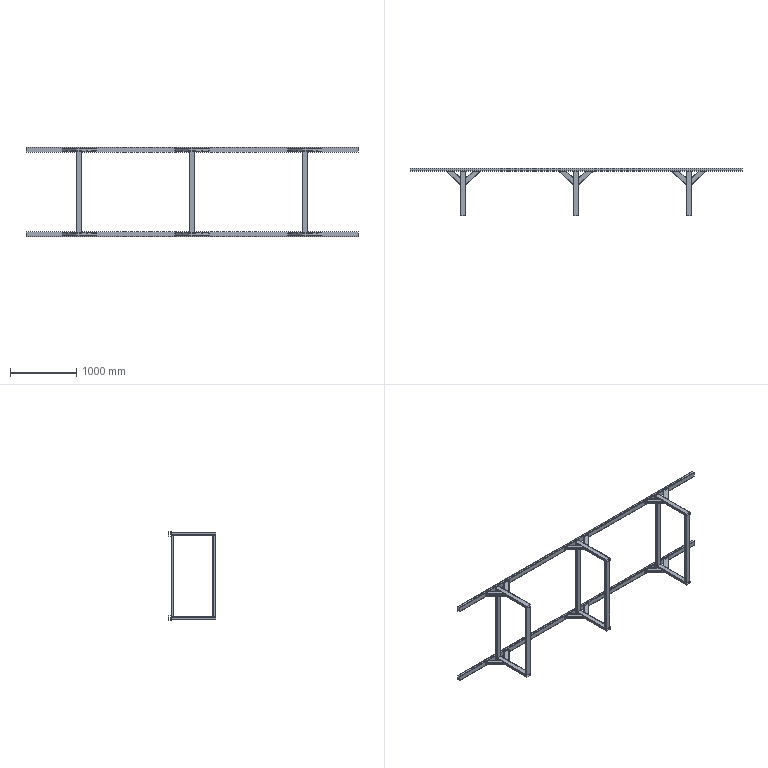Part | SolidWorks | features WeldCornerFeat 6, 3DProfileFeature 1, WeldMemberFeat 1, WeldmentFeature 1 | 26 solids | 468 faces | box 5000 x 710 x 1350 mm | volume 15935938 mm3 | plane 260 | cylinder 208 | commonest cylinder face diameters 6 x104 12 x104